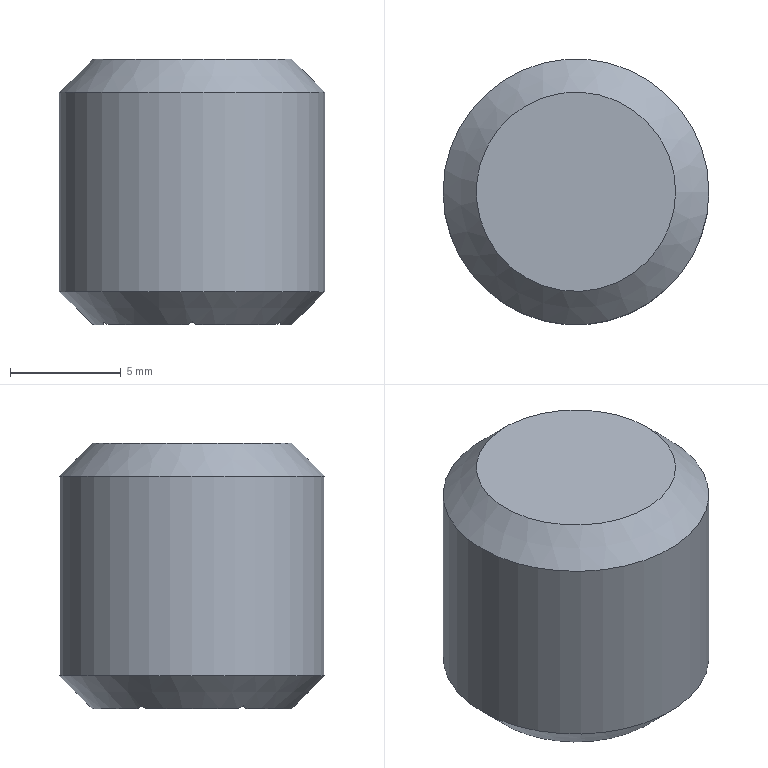Part | NX | features WTM12.00 2 | 1 solid | 17 faces | box 12 x 12 x 12 mm | volume 836.006 mm3 | plane 14 | cone 2 | cylinder 1 | commonest cylinder face diameters 12 x1
STEP:
#1=CARTESIAN_POINT('',(-101.,-82.938,-84.));
#2=VERTEX_POINT('',#1);
#3=CARTESIAN_POINT('',(-101.,-87.062,-84.));
#4=VERTEX_POINT('',#3);
#5=CARTESIAN_POINT('',(-101.,-82.691,-84.));
#6=DIRECTION('',(0.,-1.,0.));
#7=VECTOR('',#6,1000.);
#8=LINE('',#5,#7);
#9=EDGE_CURVE('',#2,#4,#8,.T.);
#10=ORIENTED_EDGE('',*,*,#9,.F.);
#11=CARTESIAN_POINT('',(-105.,-85.,-84.));
#12=DIRECTION('',(0.,0.,1.));
#13=DIRECTION('',(-1.,0.,0.));
#14=AXIS2_PLACEMENT_3D('',#11,#12,#13);
#15=CIRCLE('',#14,4.5);
#16=EDGE_CURVE('',#4,#2,#15,.T.);
#17=ORIENTED_EDGE('',*,*,#16,.F.);
#18=EDGE_LOOP('',(#10,#17));
#19=FACE_BOUND('',#18,.T.);
#20=CARTESIAN_POINT('',(-105.,-85.,-84.));
#21=DIRECTION('',(0.,0.,-1.));
#22=DIRECTION('',(-1.,0.,0.));
#23=AXIS2_PLACEMENT_3D('',#20,#21,#22);
#24=PLANE('',#23);
#25=ADVANCED_FACE('',(#19),#24,.T.);
#26=CARTESIAN_POINT('',(-104.785,-80.505,-84.));
#27=VERTEX_POINT('',#26);
#28=CARTESIAN_POINT('',(-101.215,-82.567,-84.));
#29=VERTEX_POINT('',#28);
#30=CARTESIAN_POINT('',(-105.,-80.381,-84.));
#31=DIRECTION('',(0.866,-0.5,0.));
#32=VECTOR('',#31,1000.);
#33=LINE('',#30,#32);
#34=EDGE_CURVE('',#27,#29,#33,.T.);
#35=ORIENTED_EDGE('',*,*,#34,.F.);
#36=CARTESIAN_POINT('',(-105.,-85.,-84.));
#37=DIRECTION('',(0.,0.,1.));
#38=DIRECTION('',(-1.,0.,0.));
#39=AXIS2_PLACEMENT_3D('',#36,#37,#38);
#40=CIRCLE('',#39,4.5);
#41=EDGE_CURVE('',#29,#27,#40,.T.);
#42=ORIENTED_EDGE('',*,*,#41,.F.);
#43=EDGE_LOOP('',(#35,#42));
#44=FACE_BOUND('',#43,.T.);
#45=CARTESIAN_POINT('',(-105.,-85.,-84.));
#46=DIRECTION('',(0.,0.,-1.));
#47=DIRECTION('',(-1.,0.,0.));
#48=AXIS2_PLACEMENT_3D('',#45,#46,#47);
#49=PLANE('',#48);
#50=ADVANCED_FACE('',(#44),#49,.T.);
#51=CARTESIAN_POINT('',(-108.785,-82.567,-84.));
#52=VERTEX_POINT('',#51);
#53=CARTESIAN_POINT('',(-105.215,-80.505,-84.));
#54=VERTEX_POINT('',#53);
#55=CARTESIAN_POINT('',(-109.,-82.691,-84.));
#56=DIRECTION('',(0.866,0.5,0.));
#57=VECTOR('',#56,1000.);
#58=LINE('',#55,#57);
#59=EDGE_CURVE('',#52,#54,#58,.T.);
#60=ORIENTED_EDGE('',*,*,#59,.F.);
#61=CARTESIAN_POINT('',(-105.,-85.,-84.));
#62=DIRECTION('',(0.,0.,1.));
#63=DIRECTION('',(-1.,0.,0.));
#64=AXIS2_PLACEMENT_3D('',#61,#62,#63);
#65=CIRCLE('',#64,4.5);
#66=EDGE_CURVE('',#54,#52,#65,.T.);
#67=ORIENTED_EDGE('',*,*,#66,.F.);
#68=EDGE_LOOP('',(#60,#67));
#69=FACE_BOUND('',#68,.T.);
#70=CARTESIAN_POINT('',(-105.,-85.,-84.));
#71=DIRECTION('',(0.,0.,-1.));
#72=DIRECTION('',(-1.,0.,0.));
#73=AXIS2_PLACEMENT_3D('',#70,#71,#72);
#74=PLANE('',#73);
#75=ADVANCED_FACE('',(#69),#74,.T.);
#76=CARTESIAN_POINT('',(-109.,-87.062,-84.));
#77=VERTEX_POINT('',#76);
#78=CARTESIAN_POINT('',(-109.,-82.938,-84.));
#79=VERTEX_POINT('',#78);
#80=CARTESIAN_POINT('',(-109.,-87.309,-84.));
#81=DIRECTION('',(0.,1.,0.));
#82=VECTOR('',#81,1000.);
#83=LINE('',#80,#82);
#84=EDGE_CURVE('',#77,#79,#83,.T.);
#85=ORIENTED_EDGE('',*,*,#84,.F.);
#86=CARTESIAN_POINT('',(-105.,-85.,-84.));
#87=DIRECTION('',(0.,0.,1.));
#88=DIRECTION('',(-1.,0.,0.));
#89=AXIS2_PLACEMENT_3D('',#86,#87,#88);
#90=CIRCLE('',#89,4.5);
#91=EDGE_CURVE('',#79,#77,#90,.T.);
#92=ORIENTED_EDGE('',*,*,#91,.F.);
#93=EDGE_LOOP('',(#85,#92));
#94=FACE_BOUND('',#93,.T.);
#95=CARTESIAN_POINT('',(-105.,-85.,-84.));
#96=DIRECTION('',(0.,0.,-1.));
#97=DIRECTION('',(-1.,0.,0.));
#98=AXIS2_PLACEMENT_3D('',#95,#96,#97);
#99=PLANE('',#98);
#100=ADVANCED_FACE('',(#94),#99,.T.);
#101=CARTESIAN_POINT('',(-105.215,-89.495,-84.));
#102=VERTEX_POINT('',#101);
#103=CARTESIAN_POINT('',(-108.785,-87.433,-84.));
#104=VERTEX_POINT('',#103);
#105=CARTESIAN_POINT('',(-105.,-89.619,-84.));
#106=DIRECTION('',(-0.866,0.5,0.));
#107=VECTOR('',#106,1000.);
#108=LINE('',#105,#107);
#109=EDGE_CURVE('',#102,#104,#108,.T.);
#110=ORIENTED_EDGE('',*,*,#109,.F.);
#111=CARTESIAN_POINT('',(-105.,-85.,-84.));
#112=DIRECTION('',(0.,0.,1.));
#113=DIRECTION('',(-1.,0.,0.));
#114=AXIS2_PLACEMENT_3D('',#111,#112,#113);
#115=CIRCLE('',#114,4.5);
#116=EDGE_CURVE('',#104,#102,#115,.T.);
#117=ORIENTED_EDGE('',*,*,#116,.F.);
#118=EDGE_LOOP('',(#110,#117));
#119=FACE_BOUND('',#118,.T.);
#120=CARTESIAN_POINT('',(-105.,-85.,-84.));
#121=DIRECTION('',(0.,0.,-1.));
#122=DIRECTION('',(-1.,0.,0.));
#123=AXIS2_PLACEMENT_3D('',#120,#121,#122);
#124=PLANE('',#123);
#125=ADVANCED_FACE('',(#119),#124,.T.);
#126=CARTESIAN_POINT('',(-101.215,-87.433,-84.));
#127=VERTEX_POINT('',#126);
#128=CARTESIAN_POINT('',(-104.785,-89.495,-84.));
#129=VERTEX_POINT('',#128);
#130=CARTESIAN_POINT('',(-101.,-87.309,-84.));
#131=DIRECTION('',(-0.866,-0.5,0.));
#132=VECTOR('',#131,1000.);
#133=LINE('',#130,#132);
#134=EDGE_CURVE('',#127,#129,#133,.T.);
#135=ORIENTED_EDGE('',*,*,#134,.F.);
#136=CARTESIAN_POINT('',(-105.,-85.,-84.));
#137=DIRECTION('',(0.,0.,1.));
#138=DIRECTION('',(-1.,0.,0.));
#139=AXIS2_PLACEMENT_3D('',#136,#137,#138);
#140=CIRCLE('',#139,4.5);
#141=EDGE_CURVE('',#129,#127,#140,.T.);
#142=ORIENTED_EDGE('',*,*,#141,.F.);
#143=EDGE_LOOP('',(#135,#142));
#144=FACE_BOUND('',#143,.T.);
#145=CARTESIAN_POINT('',(-105.,-85.,-84.));
#146=DIRECTION('',(0.,0.,-1.));
#147=DIRECTION('',(-1.,0.,0.));
#148=AXIS2_PLACEMENT_3D('',#145,#146,#147);
#149=PLANE('',#148);
#150=ADVANCED_FACE('',(#144),#149,.T.);
#151=CARTESIAN_POINT('',(-100.5,-85.,-72.));
#152=VERTEX_POINT('',#151);
#153=CARTESIAN_POINT('',(-105.,-85.,-72.));
#154=DIRECTION('',(0.,0.,-1.));
#155=DIRECTION('',(1.,0.,0.));
#156=AXIS2_PLACEMENT_3D('',#153,#154,#155);
#157=CIRCLE('',#156,4.5);
#158=EDGE_CURVE('',#152,#152,#157,.T.);
#159=ORIENTED_EDGE('',*,*,#158,.F.);
#160=EDGE_LOOP('',(#159));
#161=FACE_BOUND('',#160,.T.);
#162=CARTESIAN_POINT('',(-105.,-85.,-72.));
#163=DIRECTION('',(0.,0.,1.));
#164=DIRECTION('',(1.,0.,0.));
#165=AXIS2_PLACEMENT_3D('',#162,#163,#164);
#166=PLANE('',#165);
#167=ADVANCED_FACE('',(#161),#166,.T.);
#168=CARTESIAN_POINT('',(-111.,-85.,-82.5));
#169=VERTEX_POINT('',#168);
#170=CARTESIAN_POINT('',(-105.,-85.,-82.5));
#171=DIRECTION('',(0.,0.,1.));
#172=DIRECTION('',(-1.,0.,0.));
#173=AXIS2_PLACEMENT_3D('',#170,#171,#172);
#174=CIRCLE('',#173,6.);
#175=EDGE_CURVE('',#169,#169,#174,.F.);
#176=ORIENTED_EDGE('',*,*,#175,.F.);
#177=EDGE_LOOP('',(#176));
#178=FACE_BOUND('',#177,.T.);
#179=CARTESIAN_POINT('',(-99.,-85.,-73.5));
#180=VERTEX_POINT('',#179);
#181=CARTESIAN_POINT('',(-105.,-85.,-73.5));
#182=DIRECTION('',(0.,0.,-1.));
#183=DIRECTION('',(1.,0.,0.));
#184=AXIS2_PLACEMENT_3D('',#181,#182,#183);
#185=CIRCLE('',#184,6.);
#186=EDGE_CURVE('',#180,#180,#185,.F.);
#187=ORIENTED_EDGE('',*,*,#186,.F.);
#188=EDGE_LOOP('',(#187));
#189=FACE_BOUND('',#188,.T.);
#190=CARTESIAN_POINT('',(-105.,-85.,-72.));
#191=DIRECTION('',(0.,0.,-1.));
#192=DIRECTION('',(1.,0.,0.));
#193=AXIS2_PLACEMENT_3D('',#190,#191,#192);
#194=CYLINDRICAL_SURFACE('',#193,6.);
#195=ADVANCED_FACE('',(#178,#189),#194,.T.);
#196=CARTESIAN_POINT('',(-105.,-80.381,-76.));
#197=VERTEX_POINT('',#196);
#198=CARTESIAN_POINT('',(-105.,-80.381,-83.881));
#199=VERTEX_POINT('',#198);
#200=CARTESIAN_POINT('',(-105.,-80.381,-84.));
#201=DIRECTION('',(0.,0.,1.));
#202=VECTOR('',#201,1000.);
#203=LINE('',#200,#202);
#204=EDGE_CURVE('',#197,#199,#203,.F.);
#205=ORIENTED_EDGE('',*,*,#204,.F.);
#206=CARTESIAN_POINT('',(-109.,-82.691,-76.));
#207=VERTEX_POINT('',#206);
#208=CARTESIAN_POINT('',(-109.,-82.691,-76.));
#209=DIRECTION('',(0.866,0.5,0.));
#210=VECTOR('',#209,1000.);
#211=LINE('',#208,#210);
#212=EDGE_CURVE('',#197,#207,#211,.F.);
#213=ORIENTED_EDGE('',*,*,#212,.T.);
#214=CARTESIAN_POINT('',(-109.,-82.691,-83.881));
#215=VERTEX_POINT('',#214);
#216=CARTESIAN_POINT('',(-109.,-82.691,-84.));
#217=DIRECTION('',(0.,0.,1.));
#218=VECTOR('',#217,1000.);
#219=LINE('',#216,#218);
#220=EDGE_CURVE('',#207,#215,#219,.F.);
#221=ORIENTED_EDGE('',*,*,#220,.T.);
#222=CARTESIAN_POINT('',(-108.785,-82.567,-84.));
#223=CARTESIAN_POINT('',(-108.858,-82.608,-83.962));
#224=CARTESIAN_POINT('',(-108.929,-82.65,-83.922));
#225=CARTESIAN_POINT('',(-109.,-82.691,-83.881));
#226=B_SPLINE_CURVE_WITH_KNOTS('',3,(#222,#223,#224,#225),.UNSPECIFIED.,.F.,.F.,(4,4),(0.,0.0002749),.UNSPECIFIED.);
#227=EDGE_CURVE('',#52,#215,#226,.T.);
#228=ORIENTED_EDGE('',*,*,#227,.F.);
#229=ORIENTED_EDGE('',*,*,#59,.T.);
#230=CARTESIAN_POINT('',(-105.,-80.381,-83.881));
#231=CARTESIAN_POINT('',(-105.071,-80.422,-83.922));
#232=CARTESIAN_POINT('',(-105.142,-80.463,-83.962));
#233=CARTESIAN_POINT('',(-105.215,-80.505,-84.));
#234=B_SPLINE_CURVE_WITH_KNOTS('',3,(#230,#231,#232,#233),.UNSPECIFIED.,.F.,.F.,(4,4),(0.,0.0002749),.UNSPECIFIED.);
#235=EDGE_CURVE('',#199,#54,#234,.T.);
#236=ORIENTED_EDGE('',*,*,#235,.F.);
#237=EDGE_LOOP('',(#205,#213,#221,#228,#229,#236));
#238=FACE_BOUND('',#237,.T.);
#239=CARTESIAN_POINT('',(-107.,-81.536,-80.));
#240=DIRECTION('',(-0.5,0.866,0.));
#241=DIRECTION('',(0.866,0.5,0.));
#242=AXIS2_PLACEMENT_3D('',#239,#240,#241);
#243=PLANE('',#242);
#244=ADVANCED_FACE('',(#238),#243,.F.);
#245=ORIENTED_EDGE('',*,*,#220,.F.);
#246=CARTESIAN_POINT('',(-109.,-87.309,-76.));
#247=VERTEX_POINT('',#246);
#248=CARTESIAN_POINT('',(-109.,-87.309,-76.));
#249=DIRECTION('',(0.,1.,0.));
#250=VECTOR('',#249,1000.);
#251=LINE('',#248,#250);
#252=EDGE_CURVE('',#207,#247,#251,.F.);
#253=ORIENTED_EDGE('',*,*,#252,.T.);
#254=CARTESIAN_POINT('',(-109.,-87.309,-83.881));
#255=VERTEX_POINT('',#254);
#256=CARTESIAN_POINT('',(-109.,-87.309,-84.));
#257=DIRECTION('',(0.,0.,1.));
#258=VECTOR('',#257,1000.);
#259=LINE('',#256,#258);
#260=EDGE_CURVE('',#247,#255,#259,.F.);
#261=ORIENTED_EDGE('',*,*,#260,.T.);
#262=CARTESIAN_POINT('',(-109.,-87.062,-84.));
#263=CARTESIAN_POINT('',(-109.,-87.145,-83.962));
#264=CARTESIAN_POINT('',(-109.,-87.227,-83.922));
#265=CARTESIAN_POINT('',(-109.,-87.309,-83.881));
#266=B_SPLINE_CURVE_WITH_KNOTS('',3,(#262,#263,#264,#265),.UNSPECIFIED.,.F.,.F.,(4,4),(0.,0.0002749),.UNSPECIFIED.);
#267=EDGE_CURVE('',#77,#255,#266,.T.);
#268=ORIENTED_EDGE('',*,*,#267,.F.);
#269=ORIENTED_EDGE('',*,*,#84,.T.);
#270=CARTESIAN_POINT('',(-109.,-82.691,-83.881));
#271=CARTESIAN_POINT('',(-109.,-82.773,-83.922));
#272=CARTESIAN_POINT('',(-109.,-82.855,-83.962));
#273=CARTESIAN_POINT('',(-109.,-82.938,-84.));
#274=B_SPLINE_CURVE_WITH_KNOTS('',3,(#270,#271,#272,#273),.UNSPECIFIED.,.F.,.F.,(4,4),(0.,0.0002749),.UNSPECIFIED.);
#275=EDGE_CURVE('',#215,#79,#274,.T.);
#276=ORIENTED_EDGE('',*,*,#275,.F.);
#277=EDGE_LOOP('',(#245,#253,#261,#268,#269,#276));
#278=FACE_BOUND('',#277,.T.);
#279=CARTESIAN_POINT('',(-109.,-85.,-80.));
#280=DIRECTION('',(-1.,0.,0.));
#281=DIRECTION('',(0.,0.,1.));
#282=AXIS2_PLACEMENT_3D('',#279,#280,#281);
#283=PLANE('',#282);
#284=ADVANCED_FACE('',(#278),#283,.F.);
#285=ORIENTED_EDGE('',*,*,#260,.F.);
#286=CARTESIAN_POINT('',(-105.,-89.619,-76.));
#287=VERTEX_POINT('',#286);
#288=CARTESIAN_POINT('',(-105.,-89.619,-76.));
#289=DIRECTION('',(-0.866,0.5,0.));
#290=VECTOR('',#289,1000.);
#291=LINE('',#288,#290);
#292=EDGE_CURVE('',#247,#287,#291,.F.);
#293=ORIENTED_EDGE('',*,*,#292,.T.);
#294=CARTESIAN_POINT('',(-105.,-89.619,-83.881));
#295=VERTEX_POINT('',#294);
#296=CARTESIAN_POINT('',(-105.,-89.619,-84.));
#297=DIRECTION('',(0.,0.,1.));
#298=VECTOR('',#297,1000.);
#299=LINE('',#296,#298);
#300=EDGE_CURVE('',#287,#295,#299,.F.);
#301=ORIENTED_EDGE('',*,*,#300,.T.);
#302=CARTESIAN_POINT('',(-105.215,-89.495,-84.));
#303=CARTESIAN_POINT('',(-105.142,-89.537,-83.962));
#304=CARTESIAN_POINT('',(-105.071,-89.578,-83.922));
#305=CARTESIAN_POINT('',(-105.,-89.619,-83.881));
#306=B_SPLINE_CURVE_WITH_KNOTS('',3,(#302,#303,#304,#305),.UNSPECIFIED.,.F.,.F.,(4,4),(0.,0.0002749),.UNSPECIFIED.);
#307=EDGE_CURVE('',#102,#295,#306,.T.);
#308=ORIENTED_EDGE('',*,*,#307,.F.);
#309=ORIENTED_EDGE('',*,*,#109,.T.);
#310=CARTESIAN_POINT('',(-109.,-87.309,-83.881));
#311=CARTESIAN_POINT('',(-108.929,-87.35,-83.922));
#312=CARTESIAN_POINT('',(-108.858,-87.392,-83.962));
#313=CARTESIAN_POINT('',(-108.785,-87.433,-84.));
#314=B_SPLINE_CURVE_WITH_KNOTS('',3,(#310,#311,#312,#313),.UNSPECIFIED.,.F.,.F.,(4,4),(0.,0.0002749),.UNSPECIFIED.);
#315=EDGE_CURVE('',#255,#104,#314,.T.);
#316=ORIENTED_EDGE('',*,*,#315,.F.);
#317=EDGE_LOOP('',(#285,#293,#301,#308,#309,#316));
#318=FACE_BOUND('',#317,.T.);
#319=CARTESIAN_POINT('',(-107.,-88.464,-80.));
#320=DIRECTION('',(-0.5,-0.866,0.));
#321=DIRECTION('',(-0.866,0.5,0.));
#322=AXIS2_PLACEMENT_3D('',#319,#320,#321);
#323=PLANE('',#322);
#324=ADVANCED_FACE('',(#318),#323,.F.);
#325=ORIENTED_EDGE('',*,*,#300,.F.);
#326=CARTESIAN_POINT('',(-101.,-87.309,-76.));
#327=VERTEX_POINT('',#326);
#328=CARTESIAN_POINT('',(-101.,-87.309,-76.));
#329=DIRECTION('',(-0.866,-0.5,0.));
#330=VECTOR('',#329,1000.);
#331=LINE('',#328,#330);
#332=EDGE_CURVE('',#287,#327,#331,.F.);
#333=ORIENTED_EDGE('',*,*,#332,.T.);
#334=CARTESIAN_POINT('',(-101.,-87.309,-83.881));
#335=VERTEX_POINT('',#334);
#336=CARTESIAN_POINT('',(-101.,-87.309,-84.));
#337=DIRECTION('',(0.,0.,1.));
#338=VECTOR('',#337,1000.);
#339=LINE('',#336,#338);
#340=EDGE_CURVE('',#327,#335,#339,.F.);
#341=ORIENTED_EDGE('',*,*,#340,.T.);
#342=CARTESIAN_POINT('',(-101.215,-87.433,-84.));
#343=CARTESIAN_POINT('',(-101.142,-87.392,-83.962));
#344=CARTESIAN_POINT('',(-101.071,-87.35,-83.922));
#345=CARTESIAN_POINT('',(-101.,-87.309,-83.881));
#346=B_SPLINE_CURVE_WITH_KNOTS('',3,(#342,#343,#344,#345),.UNSPECIFIED.,.F.,.F.,(4,4),(0.,0.0002749),.UNSPECIFIED.);
#347=EDGE_CURVE('',#127,#335,#346,.T.);
#348=ORIENTED_EDGE('',*,*,#347,.F.);
#349=ORIENTED_EDGE('',*,*,#134,.T.);
#350=CARTESIAN_POINT('',(-105.,-89.619,-83.881));
#351=CARTESIAN_POINT('',(-104.929,-89.578,-83.922));
#352=CARTESIAN_POINT('',(-104.858,-89.537,-83.962));
#353=CARTESIAN_POINT('',(-104.785,-89.495,-84.));
#354=B_SPLINE_CURVE_WITH_KNOTS('',3,(#350,#351,#352,#353),.UNSPECIFIED.,.F.,.F.,(4,4),(0.,0.0002749),.UNSPECIFIED.);
#355=EDGE_CURVE('',#295,#129,#354,.T.);
#356=ORIENTED_EDGE('',*,*,#355,.F.);
#357=EDGE_LOOP('',(#325,#333,#341,#348,#349,#356));
#358=FACE_BOUND('',#357,.T.);
#359=CARTESIAN_POINT('',(-103.,-88.464,-80.));
#360=DIRECTION('',(0.5,-0.866,0.));
#361=DIRECTION('',(-0.866,-0.5,0.));
#362=AXIS2_PLACEMENT_3D('',#359,#360,#361);
#363=PLANE('',#362);
#364=ADVANCED_FACE('',(#358),#363,.F.);
#365=ORIENTED_EDGE('',*,*,#9,.T.);
#366=CARTESIAN_POINT('',(-101.,-87.309,-83.881));
#367=CARTESIAN_POINT('',(-101.,-87.227,-83.922));
#368=CARTESIAN_POINT('',(-101.,-87.145,-83.962));
#369=CARTESIAN_POINT('',(-101.,-87.062,-84.));
#370=B_SPLINE_CURVE_WITH_KNOTS('',3,(#366,#367,#368,#369),.UNSPECIFIED.,.F.,.F.,(4,4),(0.,0.0002749),.UNSPECIFIED.);
#371=EDGE_CURVE('',#335,#4,#370,.T.);
#372=ORIENTED_EDGE('',*,*,#371,.F.);
#373=ORIENTED_EDGE('',*,*,#340,.F.);
#374=CARTESIAN_POINT('',(-101.,-82.691,-76.));
#375=VERTEX_POINT('',#374);
#376=CARTESIAN_POINT('',(-101.,-82.691,-76.));
#377=DIRECTION('',(0.,-1.,0.));
#378=VECTOR('',#377,1000.);
#379=LINE('',#376,#378);
#380=EDGE_CURVE('',#327,#375,#379,.F.);
#381=ORIENTED_EDGE('',*,*,#380,.T.);
#382=CARTESIAN_POINT('',(-101.,-82.691,-83.881));
#383=VERTEX_POINT('',#382);
#384=CARTESIAN_POINT('',(-101.,-82.691,-84.));
#385=DIRECTION('',(0.,0.,1.));
#386=VECTOR('',#385,1000.);
#387=LINE('',#384,#386);
#388=EDGE_CURVE('',#375,#383,#387,.F.);
#389=ORIENTED_EDGE('',*,*,#388,.T.);
#390=CARTESIAN_POINT('',(-101.,-82.938,-84.));
#391=CARTESIAN_POINT('',(-101.,-82.855,-83.962));
#392=CARTESIAN_POINT('',(-101.,-82.773,-83.922));
#393=CARTESIAN_POINT('',(-101.,-82.691,-83.881));
#394=B_SPLINE_CURVE_WITH_KNOTS('',3,(#390,#391,#392,#393),.UNSPECIFIED.,.F.,.F.,(4,4),(0.,0.0002749),.UNSPECIFIED.);
#395=EDGE_CURVE('',#2,#383,#394,.T.);
#396=ORIENTED_EDGE('',*,*,#395,.F.);
#397=EDGE_LOOP('',(#365,#372,#373,#381,#389,#396));
#398=FACE_BOUND('',#397,.T.);
#399=CARTESIAN_POINT('',(-101.,-85.,-80.));
#400=DIRECTION('',(1.,0.,0.));
#401=DIRECTION('',(0.,0.,-1.));
#402=AXIS2_PLACEMENT_3D('',#399,#400,#401);
#403=PLANE('',#402);
#404=ADVANCED_FACE('',(#398),#403,.F.);
#405=ORIENTED_EDGE('',*,*,#388,.F.);
#406=CARTESIAN_POINT('',(-105.,-80.381,-76.));
#407=DIRECTION('',(0.866,-0.5,0.));
#408=VECTOR('',#407,1000.);
#409=LINE('',#406,#408);
#410=EDGE_CURVE('',#375,#197,#409,.F.);
#411=ORIENTED_EDGE('',*,*,#410,.T.);
#412=ORIENTED_EDGE('',*,*,#204,.T.);
#413=CARTESIAN_POINT('',(-104.785,-80.505,-84.));
#414=CARTESIAN_POINT('',(-104.858,-80.463,-83.962));
#415=CARTESIAN_POINT('',(-104.929,-80.422,-83.922));
#416=CARTESIAN_POINT('',(-105.,-80.381,-83.881));
#417=B_SPLINE_CURVE_WITH_KNOTS('',3,(#413,#414,#415,#416),.UNSPECIFIED.,.F.,.F.,(4,4),(0.,0.0002749),.UNSPECIFIED.);
#418=EDGE_CURVE('',#27,#199,#417,.T.);
#419=ORIENTED_EDGE('',*,*,#418,.F.);
#420=ORIENTED_EDGE('',*,*,#34,.T.);
#421=CARTESIAN_POINT('',(-101.,-82.691,-83.881));
#422=CARTESIAN_POINT('',(-101.071,-82.65,-83.922));
#423=CARTESIAN_POINT('',(-101.142,-82.608,-83.962));
#424=CARTESIAN_POINT('',(-101.215,-82.567,-84.));
#425=B_SPLINE_CURVE_WITH_KNOTS('',3,(#421,#422,#423,#424),.UNSPECIFIED.,.F.,.F.,(4,4),(0.,0.0002749),.UNSPECIFIED.);
#426=EDGE_CURVE('',#383,#29,#425,.T.);
#427=ORIENTED_EDGE('',*,*,#426,.F.);
#428=EDGE_LOOP('',(#405,#411,#412,#419,#420,#427));
#429=FACE_BOUND('',#428,.T.);
#430=CARTESIAN_POINT('',(-103.,-81.536,-80.));
#431=DIRECTION('',(0.5,0.866,0.));
#432=DIRECTION('',(0.866,-0.5,0.));
#433=AXIS2_PLACEMENT_3D('',#430,#431,#432);
#434=PLANE('',#433);
#435=ADVANCED_FACE('',(#429),#434,.F.);
#436=ORIENTED_EDGE('',*,*,#252,.F.);
#437=ORIENTED_EDGE('',*,*,#212,.F.);
#438=ORIENTED_EDGE('',*,*,#410,.F.);
#439=ORIENTED_EDGE('',*,*,#380,.F.);
#440=ORIENTED_EDGE('',*,*,#332,.F.);
#441=ORIENTED_EDGE('',*,*,#292,.F.);
#442=EDGE_LOOP('',(#436,#437,#438,#439,#440,#441));
#443=FACE_BOUND('',#442,.T.);
#444=CARTESIAN_POINT('',(-105.,-85.,-76.));
#445=DIRECTION('',(0.,0.,1.));
#446=DIRECTION('',(1.,0.,0.));
#447=AXIS2_PLACEMENT_3D('',#444,#445,#446);
#448=PLANE('',#447);
#449=ADVANCED_FACE('',(#443),#448,.F.);
#450=ORIENTED_EDGE('',*,*,#395,.T.);
#451=ORIENTED_EDGE('',*,*,#426,.T.);
#452=ORIENTED_EDGE('',*,*,#41,.T.);
#453=ORIENTED_EDGE('',*,*,#418,.T.);
#454=ORIENTED_EDGE('',*,*,#235,.T.);
#455=ORIENTED_EDGE('',*,*,#66,.T.);
#456=ORIENTED_EDGE('',*,*,#227,.T.);
#457=ORIENTED_EDGE('',*,*,#275,.T.);
#458=ORIENTED_EDGE('',*,*,#91,.T.);
#459=ORIENTED_EDGE('',*,*,#267,.T.);
#460=ORIENTED_EDGE('',*,*,#315,.T.);
#461=ORIENTED_EDGE('',*,*,#116,.T.);
#462=ORIENTED_EDGE('',*,*,#307,.T.);
#463=ORIENTED_EDGE('',*,*,#355,.T.);
#464=ORIENTED_EDGE('',*,*,#141,.T.);
#465=ORIENTED_EDGE('',*,*,#347,.T.);
#466=ORIENTED_EDGE('',*,*,#371,.T.);
#467=ORIENTED_EDGE('',*,*,#16,.T.);
#468=EDGE_LOOP('',(#450,#451,#452,#453,#454,#455,#456,#457,#458,#459,#460,#461,#462,#463,#464,#465,#466,#467));
#469=FACE_BOUND('',#468,.T.);
#470=ORIENTED_EDGE('',*,*,#175,.T.);
#471=EDGE_LOOP('',(#470));
#472=FACE_BOUND('',#471,.T.);
#473=CARTESIAN_POINT('',(-105.,-85.,-82.5));
#474=DIRECTION('',(0.,0.,1.));
#475=DIRECTION('',(1.,0.,0.));
#476=AXIS2_PLACEMENT_3D('',#473,#474,#475);
#477=CONICAL_SURFACE('',#476,6.,0.7854);
#478=ADVANCED_FACE('',(#469,#472),#477,.T.);
#479=ORIENTED_EDGE('',*,*,#158,.T.);
#480=EDGE_LOOP('',(#479));
#481=FACE_BOUND('',#480,.T.);
#482=ORIENTED_EDGE('',*,*,#186,.T.);
#483=EDGE_LOOP('',(#482));
#484=FACE_BOUND('',#483,.T.);
#485=CARTESIAN_POINT('',(-105.,-85.,-73.5));
#486=DIRECTION('',(0.,0.,-1.));
#487=DIRECTION('',(-1.,0.,0.));
#488=AXIS2_PLACEMENT_3D('',#485,#486,#487);
#489=CONICAL_SURFACE('',#488,6.,0.7854);
#490=ADVANCED_FACE('',(#481,#484),#489,.T.);
#491=CLOSED_SHELL('',(#25,#50,#75,#100,#125,#150,#167,#195,#244,#284,#324,#364,#404,#435,#449,#478,#490));
#492=MANIFOLD_SOLID_BREP('',#491);
#493=(LENGTH_UNIT()NAMED_UNIT(*)SI_UNIT(.MILLI.,.METRE.));
#494=UNCERTAINTY_MEASURE_WITH_UNIT(LENGTH_MEASURE(0.0508),#493,'','');
#495=(NAMED_UNIT(*)PLANE_ANGLE_UNIT()SI_UNIT($,.RADIAN.));
#496=(NAMED_UNIT(*)SI_UNIT($,.STERADIAN.)SOLID_ANGLE_UNIT());
#497=(GEOMETRIC_REPRESENTATION_CONTEXT(3)GLOBAL_UNCERTAINTY_ASSIGNED_CONTEXT((#494))GLOBAL_UNIT_ASSIGNED_CONTEXT((#493,#495,#496))REPRESENTATION_CONTEXT('',''));
#498=ADVANCED_BREP_SHAPE_REPRESENTATION('',(#492),#497);